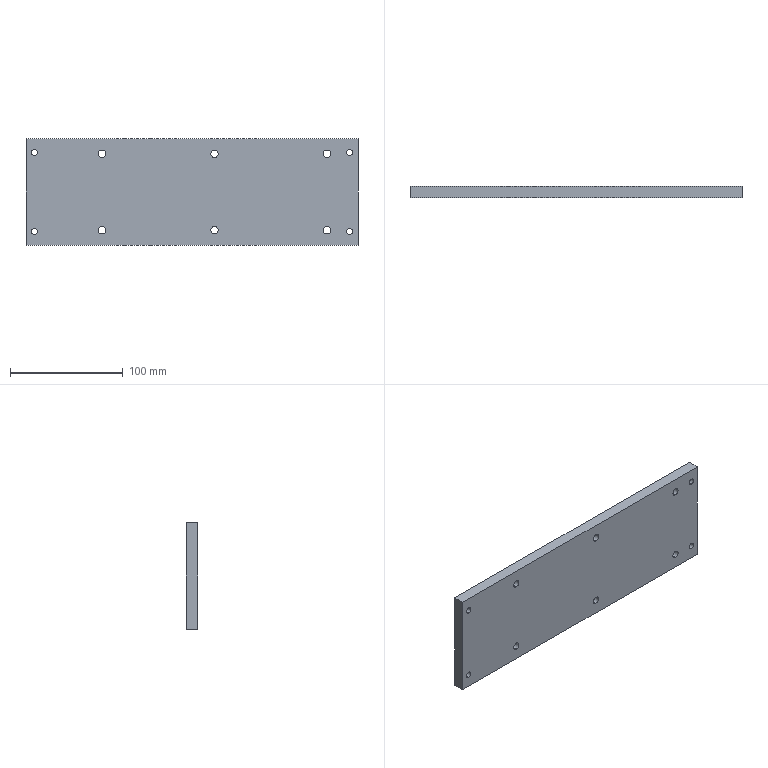Part | STEP file | Grinding bracket top plate | 1 solid | 38 faces | box 295 x 10 x 95 mm | volume 275998 mm3 | cylinder 28 | plane 10 | commonest cylinder face diameters 6.6 x12 5.5 x8 10 x8